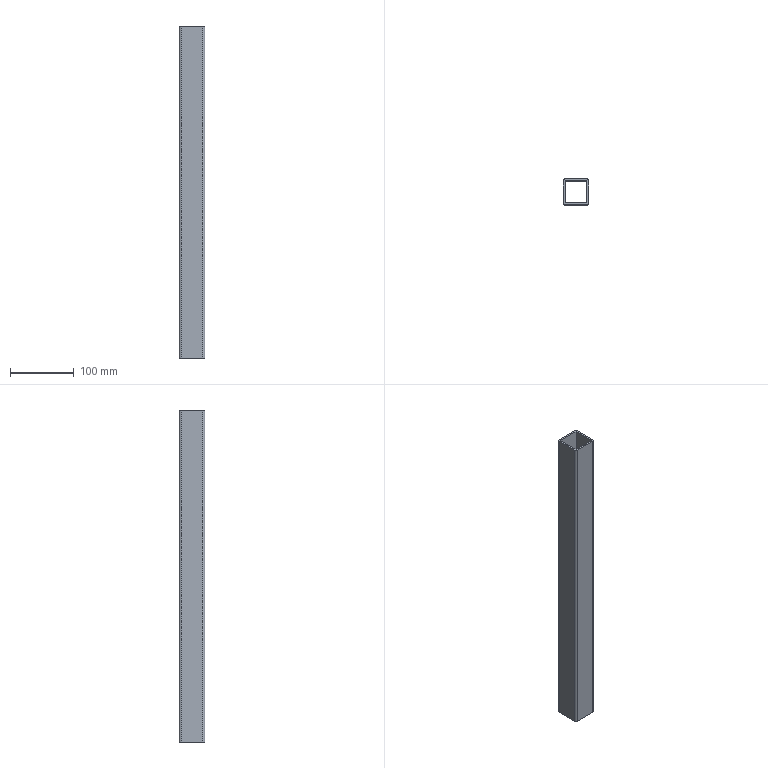Part | STEP file | X77-04202 | 1 solid | 14 faces | box 40 x 40 x 520 mm | volume 226863 mm3 | plane 10 | cylinder 4 | commonest cylinder face diameters 6 x4
STEP:
#1=CARTESIAN_POINT('',(-20.,-17.,520.));
#2=VERTEX_POINT('',#1);
#3=CARTESIAN_POINT('',(-17.,-20.,520.));
#4=VERTEX_POINT('',#3);
#5=CARTESIAN_POINT('',(-17.,-17.,520.));
#6=DIRECTION('',(0.,0.,1.));
#7=DIRECTION('',(-1.,0.,0.));
#8=AXIS2_PLACEMENT_3D('',#5,#6,#7);
#9=CIRCLE('',#8,3.);
#10=EDGE_CURVE('',#2,#4,#9,.T.);
#11=ORIENTED_EDGE('',*,*,#10,.T.);
#12=CARTESIAN_POINT('',(17.,-20.,520.));
#13=VERTEX_POINT('',#12);
#14=CARTESIAN_POINT('',(-17.,-20.,520.));
#15=DIRECTION('',(1.,0.,0.));
#16=VECTOR('',#15,1000.);
#17=LINE('',#14,#16);
#18=EDGE_CURVE('',#4,#13,#17,.T.);
#19=ORIENTED_EDGE('',*,*,#18,.T.);
#20=CARTESIAN_POINT('',(20.,-17.,520.));
#21=VERTEX_POINT('',#20);
#22=CARTESIAN_POINT('',(17.,-17.,520.));
#23=DIRECTION('',(0.,0.,1.));
#24=DIRECTION('',(-1.,0.,0.));
#25=AXIS2_PLACEMENT_3D('',#22,#23,#24);
#26=CIRCLE('',#25,3.);
#27=EDGE_CURVE('',#13,#21,#26,.T.);
#28=ORIENTED_EDGE('',*,*,#27,.T.);
#29=CARTESIAN_POINT('',(20.,17.,520.));
#30=VERTEX_POINT('',#29);
#31=CARTESIAN_POINT('',(20.,-17.,520.));
#32=DIRECTION('',(0.,1.,0.));
#33=VECTOR('',#32,1000.);
#34=LINE('',#31,#33);
#35=EDGE_CURVE('',#21,#30,#34,.T.);
#36=ORIENTED_EDGE('',*,*,#35,.T.);
#37=CARTESIAN_POINT('',(17.,20.,520.));
#38=VERTEX_POINT('',#37);
#39=CARTESIAN_POINT('',(17.,17.,520.));
#40=DIRECTION('',(0.,0.,1.));
#41=DIRECTION('',(1.,0.,0.));
#42=AXIS2_PLACEMENT_3D('',#39,#40,#41);
#43=CIRCLE('',#42,3.);
#44=EDGE_CURVE('',#30,#38,#43,.T.);
#45=ORIENTED_EDGE('',*,*,#44,.T.);
#46=CARTESIAN_POINT('',(-17.,20.,520.));
#47=VERTEX_POINT('',#46);
#48=CARTESIAN_POINT('',(-17.,20.,520.));
#49=DIRECTION('',(-1.,0.,0.));
#50=VECTOR('',#49,1000.);
#51=LINE('',#48,#50);
#52=EDGE_CURVE('',#38,#47,#51,.T.);
#53=ORIENTED_EDGE('',*,*,#52,.T.);
#54=CARTESIAN_POINT('',(-20.,17.,520.));
#55=VERTEX_POINT('',#54);
#56=CARTESIAN_POINT('',(-17.,17.,520.));
#57=DIRECTION('',(0.,0.,1.));
#58=DIRECTION('',(1.,0.,0.));
#59=AXIS2_PLACEMENT_3D('',#56,#57,#58);
#60=CIRCLE('',#59,3.);
#61=EDGE_CURVE('',#47,#55,#60,.T.);
#62=ORIENTED_EDGE('',*,*,#61,.T.);
#63=CARTESIAN_POINT('',(-20.,-17.,520.));
#64=DIRECTION('',(0.,-1.,0.));
#65=VECTOR('',#64,1000.);
#66=LINE('',#63,#65);
#67=EDGE_CURVE('',#55,#2,#66,.T.);
#68=ORIENTED_EDGE('',*,*,#67,.T.);
#69=EDGE_LOOP('',(#11,#19,#28,#36,#45,#53,#62,#68));
#70=FACE_OUTER_BOUND('',#69,.T.);
#71=CARTESIAN_POINT('',(17.,-17.,520.));
#72=VERTEX_POINT('',#71);
#73=CARTESIAN_POINT('',(17.,17.,520.));
#74=VERTEX_POINT('',#73);
#75=CARTESIAN_POINT('',(17.,-17.,520.));
#76=DIRECTION('',(0.,1.,0.));
#77=VECTOR('',#76,1000.);
#78=LINE('',#75,#77);
#79=EDGE_CURVE('',#72,#74,#78,.T.);
#80=ORIENTED_EDGE('',*,*,#79,.F.);
#81=CARTESIAN_POINT('',(-17.,-17.,520.));
#82=VERTEX_POINT('',#81);
#83=CARTESIAN_POINT('',(-17.,-17.,520.));
#84=DIRECTION('',(1.,0.,0.));
#85=VECTOR('',#84,1000.);
#86=LINE('',#83,#85);
#87=EDGE_CURVE('',#82,#72,#86,.T.);
#88=ORIENTED_EDGE('',*,*,#87,.F.);
#89=CARTESIAN_POINT('',(-17.,17.,520.));
#90=VERTEX_POINT('',#89);
#91=CARTESIAN_POINT('',(-17.,-17.,520.));
#92=DIRECTION('',(0.,-1.,0.));
#93=VECTOR('',#92,1000.);
#94=LINE('',#91,#93);
#95=EDGE_CURVE('',#90,#82,#94,.T.);
#96=ORIENTED_EDGE('',*,*,#95,.F.);
#97=CARTESIAN_POINT('',(-17.,17.,520.));
#98=DIRECTION('',(-1.,0.,0.));
#99=VECTOR('',#98,1000.);
#100=LINE('',#97,#99);
#101=EDGE_CURVE('',#74,#90,#100,.T.);
#102=ORIENTED_EDGE('',*,*,#101,.F.);
#103=EDGE_LOOP('',(#80,#88,#96,#102));
#104=FACE_BOUND('',#103,.T.);
#105=CARTESIAN_POINT('',(-17.,-17.,520.));
#106=DIRECTION('',(0.,0.,-1.));
#107=DIRECTION('',(-1.,0.,0.));
#108=AXIS2_PLACEMENT_3D('',#105,#106,#107);
#109=PLANE('',#108);
#110=ADVANCED_FACE('',(#70,#104),#109,.F.);
#111=CARTESIAN_POINT('',(-20.,-17.,0.));
#112=VERTEX_POINT('',#111);
#113=CARTESIAN_POINT('',(-17.,-20.,0.));
#114=VERTEX_POINT('',#113);
#115=CARTESIAN_POINT('',(-17.,-17.,0.));
#116=DIRECTION('',(0.,0.,1.));
#117=DIRECTION('',(-1.,0.,0.));
#118=AXIS2_PLACEMENT_3D('',#115,#116,#117);
#119=CIRCLE('',#118,3.);
#120=EDGE_CURVE('',#112,#114,#119,.T.);
#121=ORIENTED_EDGE('',*,*,#120,.F.);
#122=CARTESIAN_POINT('',(-20.,17.,0.));
#123=VERTEX_POINT('',#122);
#124=CARTESIAN_POINT('',(-20.,-17.,0.));
#125=DIRECTION('',(0.,-1.,0.));
#126=VECTOR('',#125,1000.);
#127=LINE('',#124,#126);
#128=EDGE_CURVE('',#123,#112,#127,.T.);
#129=ORIENTED_EDGE('',*,*,#128,.F.);
#130=CARTESIAN_POINT('',(-17.,20.,0.));
#131=VERTEX_POINT('',#130);
#132=CARTESIAN_POINT('',(-17.,17.,0.));
#133=DIRECTION('',(0.,0.,1.));
#134=DIRECTION('',(1.,0.,0.));
#135=AXIS2_PLACEMENT_3D('',#132,#133,#134);
#136=CIRCLE('',#135,3.);
#137=EDGE_CURVE('',#131,#123,#136,.T.);
#138=ORIENTED_EDGE('',*,*,#137,.F.);
#139=CARTESIAN_POINT('',(17.,20.,0.));
#140=VERTEX_POINT('',#139);
#141=CARTESIAN_POINT('',(-17.,20.,0.));
#142=DIRECTION('',(-1.,0.,0.));
#143=VECTOR('',#142,1000.);
#144=LINE('',#141,#143);
#145=EDGE_CURVE('',#140,#131,#144,.T.);
#146=ORIENTED_EDGE('',*,*,#145,.F.);
#147=CARTESIAN_POINT('',(20.,17.,0.));
#148=VERTEX_POINT('',#147);
#149=CARTESIAN_POINT('',(17.,17.,0.));
#150=DIRECTION('',(0.,0.,1.));
#151=DIRECTION('',(1.,0.,0.));
#152=AXIS2_PLACEMENT_3D('',#149,#150,#151);
#153=CIRCLE('',#152,3.);
#154=EDGE_CURVE('',#148,#140,#153,.T.);
#155=ORIENTED_EDGE('',*,*,#154,.F.);
#156=CARTESIAN_POINT('',(20.,-17.,0.));
#157=VERTEX_POINT('',#156);
#158=CARTESIAN_POINT('',(20.,-17.,0.));
#159=DIRECTION('',(0.,1.,0.));
#160=VECTOR('',#159,1000.);
#161=LINE('',#158,#160);
#162=EDGE_CURVE('',#157,#148,#161,.T.);
#163=ORIENTED_EDGE('',*,*,#162,.F.);
#164=CARTESIAN_POINT('',(17.,-20.,0.));
#165=VERTEX_POINT('',#164);
#166=CARTESIAN_POINT('',(17.,-17.,0.));
#167=DIRECTION('',(0.,0.,1.));
#168=DIRECTION('',(-1.,0.,0.));
#169=AXIS2_PLACEMENT_3D('',#166,#167,#168);
#170=CIRCLE('',#169,3.);
#171=EDGE_CURVE('',#165,#157,#170,.T.);
#172=ORIENTED_EDGE('',*,*,#171,.F.);
#173=CARTESIAN_POINT('',(-17.,-20.,0.));
#174=DIRECTION('',(1.,0.,0.));
#175=VECTOR('',#174,1000.);
#176=LINE('',#173,#175);
#177=EDGE_CURVE('',#114,#165,#176,.T.);
#178=ORIENTED_EDGE('',*,*,#177,.F.);
#179=EDGE_LOOP('',(#121,#129,#138,#146,#155,#163,#172,#178));
#180=FACE_OUTER_BOUND('',#179,.T.);
#181=CARTESIAN_POINT('',(-17.,-17.,0.));
#182=VERTEX_POINT('',#181);
#183=CARTESIAN_POINT('',(17.,-17.,0.));
#184=VERTEX_POINT('',#183);
#185=CARTESIAN_POINT('',(-17.,-17.,0.));
#186=DIRECTION('',(1.,0.,0.));
#187=VECTOR('',#186,1000.);
#188=LINE('',#185,#187);
#189=EDGE_CURVE('',#182,#184,#188,.T.);
#190=ORIENTED_EDGE('',*,*,#189,.T.);
#191=CARTESIAN_POINT('',(17.,17.,0.));
#192=VERTEX_POINT('',#191);
#193=CARTESIAN_POINT('',(17.,-17.,0.));
#194=DIRECTION('',(0.,1.,0.));
#195=VECTOR('',#194,1000.);
#196=LINE('',#193,#195);
#197=EDGE_CURVE('',#184,#192,#196,.T.);
#198=ORIENTED_EDGE('',*,*,#197,.T.);
#199=CARTESIAN_POINT('',(-17.,17.,0.));
#200=VERTEX_POINT('',#199);
#201=CARTESIAN_POINT('',(-17.,17.,0.));
#202=DIRECTION('',(-1.,0.,0.));
#203=VECTOR('',#202,1000.);
#204=LINE('',#201,#203);
#205=EDGE_CURVE('',#192,#200,#204,.T.);
#206=ORIENTED_EDGE('',*,*,#205,.T.);
#207=CARTESIAN_POINT('',(-17.,-17.,0.));
#208=DIRECTION('',(0.,-1.,0.));
#209=VECTOR('',#208,1000.);
#210=LINE('',#207,#209);
#211=EDGE_CURVE('',#200,#182,#210,.T.);
#212=ORIENTED_EDGE('',*,*,#211,.T.);
#213=EDGE_LOOP('',(#190,#198,#206,#212));
#214=FACE_BOUND('',#213,.T.);
#215=CARTESIAN_POINT('',(-17.,-17.,0.));
#216=DIRECTION('',(0.,0.,-1.));
#217=DIRECTION('',(-1.,0.,0.));
#218=AXIS2_PLACEMENT_3D('',#215,#216,#217);
#219=PLANE('',#218);
#220=ADVANCED_FACE('',(#180,#214),#219,.T.);
#221=ORIENTED_EDGE('',*,*,#120,.T.);
#222=CARTESIAN_POINT('',(-17.,-20.,520.));
#223=DIRECTION('',(0.,0.,-1.));
#224=VECTOR('',#223,1000.);
#225=LINE('',#222,#224);
#226=EDGE_CURVE('',#4,#114,#225,.T.);
#227=ORIENTED_EDGE('',*,*,#226,.F.);
#228=ORIENTED_EDGE('',*,*,#10,.F.);
#229=CARTESIAN_POINT('',(-20.,-17.,520.));
#230=DIRECTION('',(0.,0.,-1.));
#231=VECTOR('',#230,1000.);
#232=LINE('',#229,#231);
#233=EDGE_CURVE('',#2,#112,#232,.T.);
#234=ORIENTED_EDGE('',*,*,#233,.T.);
#235=EDGE_LOOP('',(#221,#227,#228,#234));
#236=FACE_OUTER_BOUND('',#235,.T.);
#237=CARTESIAN_POINT('',(-17.,-17.,520.));
#238=DIRECTION('',(0.,0.,-1.));
#239=DIRECTION('',(-1.,0.,0.));
#240=AXIS2_PLACEMENT_3D('',#237,#238,#239);
#241=CYLINDRICAL_SURFACE('',#240,3.);
#242=ADVANCED_FACE('',(#236),#241,.T.);
#243=ORIENTED_EDGE('',*,*,#177,.T.);
#244=CARTESIAN_POINT('',(17.,-20.,520.));
#245=DIRECTION('',(0.,0.,-1.));
#246=VECTOR('',#245,1000.);
#247=LINE('',#244,#246);
#248=EDGE_CURVE('',#13,#165,#247,.T.);
#249=ORIENTED_EDGE('',*,*,#248,.F.);
#250=ORIENTED_EDGE('',*,*,#18,.F.);
#251=ORIENTED_EDGE('',*,*,#226,.T.);
#252=EDGE_LOOP('',(#243,#249,#250,#251));
#253=FACE_OUTER_BOUND('',#252,.T.);
#254=CARTESIAN_POINT('',(-17.,-20.,520.));
#255=DIRECTION('',(0.,1.,0.));
#256=DIRECTION('',(0.,0.,1.));
#257=AXIS2_PLACEMENT_3D('',#254,#255,#256);
#258=PLANE('',#257);
#259=ADVANCED_FACE('',(#253),#258,.F.);
#260=ORIENTED_EDGE('',*,*,#171,.T.);
#261=CARTESIAN_POINT('',(20.,-17.,520.));
#262=DIRECTION('',(0.,0.,-1.));
#263=VECTOR('',#262,1000.);
#264=LINE('',#261,#263);
#265=EDGE_CURVE('',#21,#157,#264,.T.);
#266=ORIENTED_EDGE('',*,*,#265,.F.);
#267=ORIENTED_EDGE('',*,*,#27,.F.);
#268=ORIENTED_EDGE('',*,*,#248,.T.);
#269=EDGE_LOOP('',(#260,#266,#267,#268));
#270=FACE_OUTER_BOUND('',#269,.T.);
#271=CARTESIAN_POINT('',(17.,-17.,520.));
#272=DIRECTION('',(0.,0.,-1.));
#273=DIRECTION('',(-1.,0.,0.));
#274=AXIS2_PLACEMENT_3D('',#271,#272,#273);
#275=CYLINDRICAL_SURFACE('',#274,3.);
#276=ADVANCED_FACE('',(#270),#275,.T.);
#277=ORIENTED_EDGE('',*,*,#162,.T.);
#278=CARTESIAN_POINT('',(20.,17.,520.));
#279=DIRECTION('',(0.,0.,-1.));
#280=VECTOR('',#279,1000.);
#281=LINE('',#278,#280);
#282=EDGE_CURVE('',#30,#148,#281,.T.);
#283=ORIENTED_EDGE('',*,*,#282,.F.);
#284=ORIENTED_EDGE('',*,*,#35,.F.);
#285=ORIENTED_EDGE('',*,*,#265,.T.);
#286=EDGE_LOOP('',(#277,#283,#284,#285));
#287=FACE_OUTER_BOUND('',#286,.T.);
#288=CARTESIAN_POINT('',(20.,-17.,520.));
#289=DIRECTION('',(-1.,0.,0.));
#290=DIRECTION('',(0.,0.,1.));
#291=AXIS2_PLACEMENT_3D('',#288,#289,#290);
#292=PLANE('',#291);
#293=ADVANCED_FACE('',(#287),#292,.F.);
#294=ORIENTED_EDGE('',*,*,#154,.T.);
#295=CARTESIAN_POINT('',(17.,20.,520.));
#296=DIRECTION('',(0.,0.,-1.));
#297=VECTOR('',#296,1000.);
#298=LINE('',#295,#297);
#299=EDGE_CURVE('',#38,#140,#298,.T.);
#300=ORIENTED_EDGE('',*,*,#299,.F.);
#301=ORIENTED_EDGE('',*,*,#44,.F.);
#302=ORIENTED_EDGE('',*,*,#282,.T.);
#303=EDGE_LOOP('',(#294,#300,#301,#302));
#304=FACE_OUTER_BOUND('',#303,.T.);
#305=CARTESIAN_POINT('',(17.,17.,520.));
#306=DIRECTION('',(0.,0.,-1.));
#307=DIRECTION('',(-1.,0.,0.));
#308=AXIS2_PLACEMENT_3D('',#305,#306,#307);
#309=CYLINDRICAL_SURFACE('',#308,3.);
#310=ADVANCED_FACE('',(#304),#309,.T.);
#311=ORIENTED_EDGE('',*,*,#145,.T.);
#312=CARTESIAN_POINT('',(-17.,20.,520.));
#313=DIRECTION('',(0.,0.,-1.));
#314=VECTOR('',#313,1000.);
#315=LINE('',#312,#314);
#316=EDGE_CURVE('',#47,#131,#315,.T.);
#317=ORIENTED_EDGE('',*,*,#316,.F.);
#318=ORIENTED_EDGE('',*,*,#52,.F.);
#319=ORIENTED_EDGE('',*,*,#299,.T.);
#320=EDGE_LOOP('',(#311,#317,#318,#319));
#321=FACE_OUTER_BOUND('',#320,.T.);
#322=CARTESIAN_POINT('',(-17.,20.,520.));
#323=DIRECTION('',(0.,-1.,0.));
#324=DIRECTION('',(0.,0.,-1.));
#325=AXIS2_PLACEMENT_3D('',#322,#323,#324);
#326=PLANE('',#325);
#327=ADVANCED_FACE('',(#321),#326,.F.);
#328=ORIENTED_EDGE('',*,*,#137,.T.);
#329=CARTESIAN_POINT('',(-20.,17.,520.));
#330=DIRECTION('',(0.,0.,-1.));
#331=VECTOR('',#330,1000.);
#332=LINE('',#329,#331);
#333=EDGE_CURVE('',#55,#123,#332,.T.);
#334=ORIENTED_EDGE('',*,*,#333,.F.);
#335=ORIENTED_EDGE('',*,*,#61,.F.);
#336=ORIENTED_EDGE('',*,*,#316,.T.);
#337=EDGE_LOOP('',(#328,#334,#335,#336));
#338=FACE_OUTER_BOUND('',#337,.T.);
#339=CARTESIAN_POINT('',(-17.,17.,520.));
#340=DIRECTION('',(0.,0.,-1.));
#341=DIRECTION('',(-1.,0.,0.));
#342=AXIS2_PLACEMENT_3D('',#339,#340,#341);
#343=CYLINDRICAL_SURFACE('',#342,3.);
#344=ADVANCED_FACE('',(#338),#343,.T.);
#345=ORIENTED_EDGE('',*,*,#128,.T.);
#346=ORIENTED_EDGE('',*,*,#233,.F.);
#347=ORIENTED_EDGE('',*,*,#67,.F.);
#348=ORIENTED_EDGE('',*,*,#333,.T.);
#349=EDGE_LOOP('',(#345,#346,#347,#348));
#350=FACE_OUTER_BOUND('',#349,.T.);
#351=CARTESIAN_POINT('',(-20.,-17.,520.));
#352=DIRECTION('',(1.,0.,0.));
#353=DIRECTION('',(0.,0.,-1.));
#354=AXIS2_PLACEMENT_3D('',#351,#352,#353);
#355=PLANE('',#354);
#356=ADVANCED_FACE('',(#350),#355,.F.);
#357=ORIENTED_EDGE('',*,*,#197,.F.);
#358=CARTESIAN_POINT('',(17.,-17.,520.));
#359=DIRECTION('',(0.,0.,-1.));
#360=VECTOR('',#359,1000.);
#361=LINE('',#358,#360);
#362=EDGE_CURVE('',#72,#184,#361,.T.);
#363=ORIENTED_EDGE('',*,*,#362,.F.);
#364=ORIENTED_EDGE('',*,*,#79,.T.);
#365=CARTESIAN_POINT('',(17.,17.,520.));
#366=DIRECTION('',(0.,0.,-1.));
#367=VECTOR('',#366,1000.);
#368=LINE('',#365,#367);
#369=EDGE_CURVE('',#74,#192,#368,.T.);
#370=ORIENTED_EDGE('',*,*,#369,.T.);
#371=EDGE_LOOP('',(#357,#363,#364,#370));
#372=FACE_OUTER_BOUND('',#371,.T.);
#373=CARTESIAN_POINT('',(17.,-17.,520.));
#374=DIRECTION('',(-1.,0.,0.));
#375=DIRECTION('',(0.,0.,1.));
#376=AXIS2_PLACEMENT_3D('',#373,#374,#375);
#377=PLANE('',#376);
#378=ADVANCED_FACE('',(#372),#377,.T.);
#379=ORIENTED_EDGE('',*,*,#205,.F.);
#380=ORIENTED_EDGE('',*,*,#369,.F.);
#381=ORIENTED_EDGE('',*,*,#101,.T.);
#382=CARTESIAN_POINT('',(-17.,17.,520.));
#383=DIRECTION('',(0.,0.,-1.));
#384=VECTOR('',#383,1000.);
#385=LINE('',#382,#384);
#386=EDGE_CURVE('',#90,#200,#385,.T.);
#387=ORIENTED_EDGE('',*,*,#386,.T.);
#388=EDGE_LOOP('',(#379,#380,#381,#387));
#389=FACE_OUTER_BOUND('',#388,.T.);
#390=CARTESIAN_POINT('',(-17.,17.,520.));
#391=DIRECTION('',(0.,-1.,0.));
#392=DIRECTION('',(0.,0.,-1.));
#393=AXIS2_PLACEMENT_3D('',#390,#391,#392);
#394=PLANE('',#393);
#395=ADVANCED_FACE('',(#389),#394,.T.);
#396=ORIENTED_EDGE('',*,*,#211,.F.);
#397=ORIENTED_EDGE('',*,*,#386,.F.);
#398=ORIENTED_EDGE('',*,*,#95,.T.);
#399=CARTESIAN_POINT('',(-17.,-17.,520.));
#400=DIRECTION('',(0.,0.,-1.));
#401=VECTOR('',#400,1000.);
#402=LINE('',#399,#401);
#403=EDGE_CURVE('',#82,#182,#402,.T.);
#404=ORIENTED_EDGE('',*,*,#403,.T.);
#405=EDGE_LOOP('',(#396,#397,#398,#404));
#406=FACE_OUTER_BOUND('',#405,.T.);
#407=CARTESIAN_POINT('',(-17.,-17.,520.));
#408=DIRECTION('',(1.,0.,0.));
#409=DIRECTION('',(0.,0.,-1.));
#410=AXIS2_PLACEMENT_3D('',#407,#408,#409);
#411=PLANE('',#410);
#412=ADVANCED_FACE('',(#406),#411,.T.);
#413=ORIENTED_EDGE('',*,*,#189,.F.);
#414=ORIENTED_EDGE('',*,*,#403,.F.);
#415=ORIENTED_EDGE('',*,*,#87,.T.);
#416=ORIENTED_EDGE('',*,*,#362,.T.);
#417=EDGE_LOOP('',(#413,#414,#415,#416));
#418=FACE_OUTER_BOUND('',#417,.T.);
#419=CARTESIAN_POINT('',(-17.,-17.,520.));
#420=DIRECTION('',(0.,1.,0.));
#421=DIRECTION('',(0.,0.,1.));
#422=AXIS2_PLACEMENT_3D('',#419,#420,#421);
#423=PLANE('',#422);
#424=ADVANCED_FACE('',(#418),#423,.T.);
#425=CLOSED_SHELL('',(#110,#220,#242,#259,#276,#293,#310,#327,#344,#356,#378,#395,#412,#424));
#426=MANIFOLD_SOLID_BREP('',#425);
#427=CARTESIAN_POINT('',(0.,0.,0.));
#428=DIRECTION('',(0.,0.,1.));
#429=DIRECTION('',(1.,0.,0.));
#430=AXIS2_PLACEMENT_3D('',#427,#428,#429);
#431=(LENGTH_UNIT()NAMED_UNIT(*)SI_UNIT(.MILLI.,.METRE.));
#432=UNCERTAINTY_MEASURE_WITH_UNIT(LENGTH_MEASURE(0.00001),#431,'','');
#433=(NAMED_UNIT(*)PLANE_ANGLE_UNIT()SI_UNIT($,.RADIAN.));
#434=(NAMED_UNIT(*)SI_UNIT($,.STERADIAN.)SOLID_ANGLE_UNIT());
#435=(GEOMETRIC_REPRESENTATION_CONTEXT(3)GLOBAL_UNCERTAINTY_ASSIGNED_CONTEXT((#432))GLOBAL_UNIT_ASSIGNED_CONTEXT((#431,#433,#434))REPRESENTATION_CONTEXT('',''));
#436=ADVANCED_BREP_SHAPE_REPRESENTATION('',(#426,#430),#435);